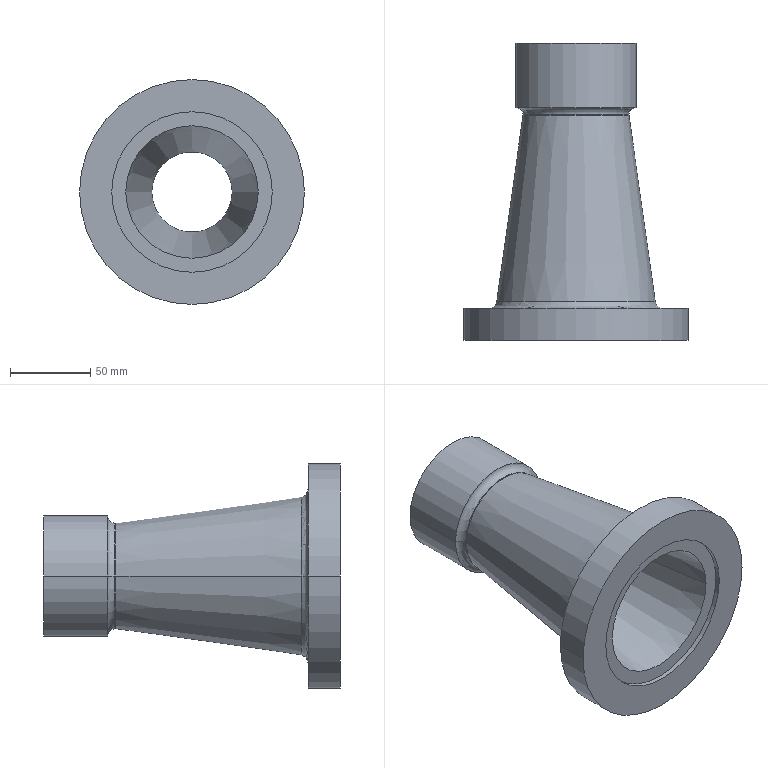Part | SolidWorks | features Revolution 1 | 1 solid | 22 faces | box 140 x 185 x 140 mm | volume 602194 mm3 | cylinder 8 | torus 6 | cone 4 | plane 4 | commonest cylinder face diameters 50 x2 75 x2 100 x2 140 x2
STEP:
#1=CARTESIAN_POINT('',(-37.5,52.5,0.));
#2=VERTEX_POINT('',#1);
#3=CARTESIAN_POINT('',(-33.,48.,0.));
#4=VERTEX_POINT('',#3);
#5=CARTESIAN_POINT('',(-37.5,48.,0.));
#6=DIRECTION('',(0.,0.,-1.));
#7=DIRECTION('',(-1.,0.,0.));
#8=AXIS2_PLACEMENT_3D('',#5,#6,#7);
#9=CIRCLE('',#8,4.5);
#10=EDGE_CURVE('',#2,#4,#9,.T.);
#11=ORIENTED_EDGE('',*,*,#10,.T.);
#12=CARTESIAN_POINT('',(33.,48.,0.));
#13=VERTEX_POINT('',#12);
#14=CARTESIAN_POINT('',(0.,48.,0.));
#15=DIRECTION('',(0.,1.,0.));
#16=DIRECTION('',(-1.,0.,0.));
#17=AXIS2_PLACEMENT_3D('',#14,#15,#16);
#18=CIRCLE('',#17,33.);
#19=EDGE_CURVE('',#4,#13,#18,.T.);
#20=ORIENTED_EDGE('',*,*,#19,.T.);
#21=CARTESIAN_POINT('',(37.5,52.5,0.));
#22=VERTEX_POINT('',#21);
#23=CARTESIAN_POINT('',(37.5,48.,0.));
#24=DIRECTION('',(0.,0.,1.));
#25=DIRECTION('',(1.,0.,0.));
#26=AXIS2_PLACEMENT_3D('',#23,#24,#25);
#27=CIRCLE('',#26,4.5);
#28=EDGE_CURVE('',#22,#13,#27,.T.);
#29=ORIENTED_EDGE('',*,*,#28,.F.);
#30=CARTESIAN_POINT('',(0.,52.5,0.));
#31=DIRECTION('',(0.,1.,0.));
#32=DIRECTION('',(-1.,0.,0.));
#33=AXIS2_PLACEMENT_3D('',#30,#31,#32);
#34=CIRCLE('',#33,37.5);
#35=EDGE_CURVE('',#2,#22,#34,.T.);
#36=ORIENTED_EDGE('',*,*,#35,.F.);
#37=EDGE_LOOP('',(#11,#20,#29,#36));
#38=FACE_OUTER_BOUND('',#37,.T.);
#39=CARTESIAN_POINT('',(0.,48.,0.));
#40=DIRECTION('',(0.,1.,0.));
#41=DIRECTION('',(-1.,0.,0.));
#42=AXIS2_PLACEMENT_3D('',#39,#40,#41);
#43=TOROIDAL_SURFACE('',#42,37.5,4.5);
#44=ADVANCED_FACE('',(#38),#43,.F.);
#45=ORIENTED_EDGE('',*,*,#28,.T.);
#46=CARTESIAN_POINT('',(0.,48.,0.));
#47=DIRECTION('',(0.,1.,0.));
#48=DIRECTION('',(-1.,0.,0.));
#49=AXIS2_PLACEMENT_3D('',#46,#47,#48);
#50=CIRCLE('',#49,33.);
#51=EDGE_CURVE('',#13,#4,#50,.T.);
#52=ORIENTED_EDGE('',*,*,#51,.T.);
#53=ORIENTED_EDGE('',*,*,#10,.F.);
#54=CARTESIAN_POINT('',(0.,52.5,0.));
#55=DIRECTION('',(0.,1.,0.));
#56=DIRECTION('',(-1.,0.,0.));
#57=AXIS2_PLACEMENT_3D('',#54,#55,#56);
#58=CIRCLE('',#57,37.5);
#59=EDGE_CURVE('',#22,#2,#58,.T.);
#60=ORIENTED_EDGE('',*,*,#59,.F.);
#61=EDGE_LOOP('',(#45,#52,#53,#60));
#62=FACE_OUTER_BOUND('',#61,.T.);
#63=CARTESIAN_POINT('',(0.,48.,0.));
#64=DIRECTION('',(0.,1.,0.));
#65=DIRECTION('',(-1.,0.,0.));
#66=AXIS2_PLACEMENT_3D('',#63,#64,#65);
#67=TOROIDAL_SURFACE('',#66,37.5,4.5);
#68=ADVANCED_FACE('',(#62),#67,.F.);
#69=ORIENTED_EDGE('',*,*,#51,.F.);
#70=CARTESIAN_POINT('',(33.044,47.37,0.));
#71=VERTEX_POINT('',#70);
#72=CARTESIAN_POINT('',(37.5,48.,0.));
#73=DIRECTION('',(0.,0.,1.));
#74=DIRECTION('',(1.,0.,0.));
#75=AXIS2_PLACEMENT_3D('',#72,#73,#74);
#76=CIRCLE('',#75,4.5);
#77=EDGE_CURVE('',#13,#71,#76,.T.);
#78=ORIENTED_EDGE('',*,*,#77,.T.);
#79=CARTESIAN_POINT('',(-33.044,47.37,0.));
#80=VERTEX_POINT('',#79);
#81=CARTESIAN_POINT('',(0.,47.37,0.));
#82=DIRECTION('',(0.,1.,0.));
#83=DIRECTION('',(-1.,0.,0.));
#84=AXIS2_PLACEMENT_3D('',#81,#82,#83);
#85=CIRCLE('',#84,33.044);
#86=EDGE_CURVE('',#71,#80,#85,.T.);
#87=ORIENTED_EDGE('',*,*,#86,.T.);
#88=CARTESIAN_POINT('',(-37.5,48.,0.));
#89=DIRECTION('',(0.,0.,-1.));
#90=DIRECTION('',(-1.,0.,0.));
#91=AXIS2_PLACEMENT_3D('',#88,#89,#90);
#92=CIRCLE('',#91,4.5);
#93=EDGE_CURVE('',#4,#80,#92,.T.);
#94=ORIENTED_EDGE('',*,*,#93,.F.);
#95=EDGE_LOOP('',(#69,#78,#87,#94));
#96=FACE_OUTER_BOUND('',#95,.T.);
#97=CARTESIAN_POINT('',(0.,48.,0.));
#98=DIRECTION('',(0.,1.,0.));
#99=DIRECTION('',(-1.,0.,0.));
#100=AXIS2_PLACEMENT_3D('',#97,#98,#99);
#101=TOROIDAL_SURFACE('',#100,37.5,4.5);
#102=ADVANCED_FACE('',(#96),#101,.F.);
#103=CARTESIAN_POINT('',(0.,47.37,0.));
#104=DIRECTION('',(0.,1.,0.));
#105=DIRECTION('',(-1.,0.,0.));
#106=AXIS2_PLACEMENT_3D('',#103,#104,#105);
#107=CIRCLE('',#106,33.044);
#108=EDGE_CURVE('',#80,#71,#107,.T.);
#109=ORIENTED_EDGE('',*,*,#108,.F.);
#110=CARTESIAN_POINT('',(-49.392,-68.2,0.));
#111=VERTEX_POINT('',#110);
#112=CARTESIAN_POINT('',(-49.392,-68.2,0.));
#113=DIRECTION('',(-0.1401,-0.9901,0.));
#114=VECTOR('',#113,1000.);
#115=LINE('',#112,#114);
#116=EDGE_CURVE('',#80,#111,#115,.T.);
#117=ORIENTED_EDGE('',*,*,#116,.T.);
#118=CARTESIAN_POINT('',(49.392,-68.2,0.));
#119=VERTEX_POINT('',#118);
#120=CARTESIAN_POINT('',(0.,-68.2,0.));
#121=DIRECTION('',(0.,1.,0.));
#122=DIRECTION('',(-1.,0.,0.));
#123=AXIS2_PLACEMENT_3D('',#120,#121,#122);
#124=CIRCLE('',#123,49.392);
#125=EDGE_CURVE('',#111,#119,#124,.T.);
#126=ORIENTED_EDGE('',*,*,#125,.T.);
#127=CARTESIAN_POINT('',(49.392,-68.2,0.));
#128=DIRECTION('',(0.1401,-0.9901,0.));
#129=VECTOR('',#128,1000.);
#130=LINE('',#127,#129);
#131=EDGE_CURVE('',#71,#119,#130,.T.);
#132=ORIENTED_EDGE('',*,*,#131,.F.);
#133=EDGE_LOOP('',(#109,#117,#126,#132));
#134=FACE_OUTER_BOUND('',#133,.T.);
#135=CARTESIAN_POINT('',(0.,-68.2,0.));
#136=DIRECTION('',(0.,-1.,0.));
#137=DIRECTION('',(1.,0.,0.));
#138=AXIS2_PLACEMENT_3D('',#135,#136,#137);
#139=CONICAL_SURFACE('',#138,49.392,0.1405);
#140=ADVANCED_FACE('',(#134),#139,.T.);
#141=CARTESIAN_POINT('',(0.,-68.2,0.));
#142=DIRECTION('',(0.,1.,0.));
#143=DIRECTION('',(-1.,0.,0.));
#144=AXIS2_PLACEMENT_3D('',#141,#142,#143);
#145=CIRCLE('',#144,49.392);
#146=EDGE_CURVE('',#119,#111,#145,.T.);
#147=ORIENTED_EDGE('',*,*,#146,.F.);
#148=CARTESIAN_POINT('',(54.343,-72.5,0.));
#149=VERTEX_POINT('',#148);
#150=CARTESIAN_POINT('',(54.343,-67.5,0.));
#151=DIRECTION('',(0.,0.,1.));
#152=DIRECTION('',(1.,0.,0.));
#153=AXIS2_PLACEMENT_3D('',#150,#151,#152);
#154=CIRCLE('',#153,5.);
#155=EDGE_CURVE('',#119,#149,#154,.T.);
#156=ORIENTED_EDGE('',*,*,#155,.T.);
#157=CARTESIAN_POINT('',(-54.343,-72.5,0.));
#158=VERTEX_POINT('',#157);
#159=CARTESIAN_POINT('',(0.,-72.5,0.));
#160=DIRECTION('',(0.,1.,0.));
#161=DIRECTION('',(-1.,0.,0.));
#162=AXIS2_PLACEMENT_3D('',#159,#160,#161);
#163=CIRCLE('',#162,54.343);
#164=EDGE_CURVE('',#149,#158,#163,.T.);
#165=ORIENTED_EDGE('',*,*,#164,.T.);
#166=CARTESIAN_POINT('',(-54.343,-67.5,0.));
#167=DIRECTION('',(0.,0.,-1.));
#168=DIRECTION('',(-1.,0.,0.));
#169=AXIS2_PLACEMENT_3D('',#166,#167,#168);
#170=CIRCLE('',#169,5.);
#171=EDGE_CURVE('',#111,#158,#170,.T.);
#172=ORIENTED_EDGE('',*,*,#171,.F.);
#173=EDGE_LOOP('',(#147,#156,#165,#172));
#174=FACE_OUTER_BOUND('',#173,.T.);
#175=CARTESIAN_POINT('',(0.,-67.5,0.));
#176=DIRECTION('',(0.,1.,0.));
#177=DIRECTION('',(-1.,0.,0.));
#178=AXIS2_PLACEMENT_3D('',#175,#176,#177);
#179=TOROIDAL_SURFACE('',#178,54.343,5.);
#180=ADVANCED_FACE('',(#174),#179,.F.);
#181=CARTESIAN_POINT('',(-70.,-92.5,0.));
#182=VERTEX_POINT('',#181);
#183=CARTESIAN_POINT('',(70.,-92.5,0.));
#184=VERTEX_POINT('',#183);
#185=CARTESIAN_POINT('',(0.,-92.5,0.));
#186=DIRECTION('',(0.,1.,0.));
#187=DIRECTION('',(-1.,0.,0.));
#188=AXIS2_PLACEMENT_3D('',#185,#186,#187);
#189=CIRCLE('',#188,70.);
#190=EDGE_CURVE('',#182,#184,#189,.T.);
#191=ORIENTED_EDGE('',*,*,#190,.T.);
#192=CARTESIAN_POINT('',(70.,-72.5,0.));
#193=VERTEX_POINT('',#192);
#194=CARTESIAN_POINT('',(70.,92.5,0.));
#195=DIRECTION('',(0.,1.,0.));
#196=VECTOR('',#195,1000.);
#197=LINE('',#194,#196);
#198=EDGE_CURVE('',#184,#193,#197,.T.);
#199=ORIENTED_EDGE('',*,*,#198,.T.);
#200=CARTESIAN_POINT('',(-70.,-72.5,0.));
#201=VERTEX_POINT('',#200);
#202=CARTESIAN_POINT('',(0.,-72.5,0.));
#203=DIRECTION('',(0.,1.,0.));
#204=DIRECTION('',(-1.,0.,0.));
#205=AXIS2_PLACEMENT_3D('',#202,#203,#204);
#206=CIRCLE('',#205,70.);
#207=EDGE_CURVE('',#201,#193,#206,.T.);
#208=ORIENTED_EDGE('',*,*,#207,.F.);
#209=CARTESIAN_POINT('',(-70.,92.5,0.));
#210=DIRECTION('',(0.,1.,0.));
#211=VECTOR('',#210,1000.);
#212=LINE('',#209,#211);
#213=EDGE_CURVE('',#182,#201,#212,.T.);
#214=ORIENTED_EDGE('',*,*,#213,.F.);
#215=EDGE_LOOP('',(#191,#199,#208,#214));
#216=FACE_OUTER_BOUND('',#215,.T.);
#217=CARTESIAN_POINT('',(0.,92.5,0.));
#218=DIRECTION('',(0.,1.,0.));
#219=DIRECTION('',(-1.,0.,0.));
#220=AXIS2_PLACEMENT_3D('',#217,#218,#219);
#221=CYLINDRICAL_SURFACE('',#220,70.);
#222=ADVANCED_FACE('',(#216),#221,.T.);
#223=CARTESIAN_POINT('',(50.,-92.5,0.));
#224=VERTEX_POINT('',#223);
#225=CARTESIAN_POINT('',(-50.,-92.5,0.));
#226=VERTEX_POINT('',#225);
#227=CARTESIAN_POINT('',(0.,-92.5,0.));
#228=DIRECTION('',(0.,1.,0.));
#229=DIRECTION('',(-1.,0.,0.));
#230=AXIS2_PLACEMENT_3D('',#227,#228,#229);
#231=CIRCLE('',#230,50.);
#232=EDGE_CURVE('',#224,#226,#231,.T.);
#233=ORIENTED_EDGE('',*,*,#232,.F.);
#234=CARTESIAN_POINT('',(50.,-89.5,0.));
#235=VERTEX_POINT('',#234);
#236=CARTESIAN_POINT('',(50.,92.5,0.));
#237=DIRECTION('',(0.,1.,0.));
#238=VECTOR('',#237,1000.);
#239=LINE('',#236,#238);
#240=EDGE_CURVE('',#224,#235,#239,.T.);
#241=ORIENTED_EDGE('',*,*,#240,.T.);
#242=CARTESIAN_POINT('',(-50.,-89.5,0.));
#243=VERTEX_POINT('',#242);
#244=CARTESIAN_POINT('',(0.,-89.5,0.));
#245=DIRECTION('',(0.,1.,0.));
#246=DIRECTION('',(-1.,0.,0.));
#247=AXIS2_PLACEMENT_3D('',#244,#245,#246);
#248=CIRCLE('',#247,50.);
#249=EDGE_CURVE('',#235,#243,#248,.T.);
#250=ORIENTED_EDGE('',*,*,#249,.T.);
#251=CARTESIAN_POINT('',(-50.,92.5,0.));
#252=DIRECTION('',(0.,1.,0.));
#253=VECTOR('',#252,1000.);
#254=LINE('',#251,#253);
#255=EDGE_CURVE('',#226,#243,#254,.T.);
#256=ORIENTED_EDGE('',*,*,#255,.F.);
#257=EDGE_LOOP('',(#233,#241,#250,#256));
#258=FACE_OUTER_BOUND('',#257,.T.);
#259=CARTESIAN_POINT('',(0.,92.5,0.));
#260=DIRECTION('',(0.,1.,0.));
#261=DIRECTION('',(-1.,0.,0.));
#262=AXIS2_PLACEMENT_3D('',#259,#260,#261);
#263=CYLINDRICAL_SURFACE('',#262,50.);
#264=ADVANCED_FACE('',(#258),#263,.F.);
#265=CARTESIAN_POINT('',(25.,25.7,0.));
#266=VERTEX_POINT('',#265);
#267=CARTESIAN_POINT('',(-25.,25.7,0.));
#268=VERTEX_POINT('',#267);
#269=CARTESIAN_POINT('',(0.,25.7,0.));
#270=DIRECTION('',(0.,1.,0.));
#271=DIRECTION('',(-1.,0.,0.));
#272=AXIS2_PLACEMENT_3D('',#269,#270,#271);
#273=CIRCLE('',#272,25.);
#274=EDGE_CURVE('',#266,#268,#273,.T.);
#275=ORIENTED_EDGE('',*,*,#274,.T.);
#276=CARTESIAN_POINT('',(-41.295,-89.5,0.));
#277=VERTEX_POINT('',#276);
#278=CARTESIAN_POINT('',(-25.,25.7,0.));
#279=DIRECTION('',(-0.1401,-0.9901,0.));
#280=VECTOR('',#279,1000.);
#281=LINE('',#278,#280);
#282=EDGE_CURVE('',#268,#277,#281,.T.);
#283=ORIENTED_EDGE('',*,*,#282,.T.);
#284=CARTESIAN_POINT('',(41.295,-89.5,0.));
#285=VERTEX_POINT('',#284);
#286=CARTESIAN_POINT('',(0.,-89.5,0.));
#287=DIRECTION('',(0.,1.,0.));
#288=DIRECTION('',(-1.,0.,0.));
#289=AXIS2_PLACEMENT_3D('',#286,#287,#288);
#290=CIRCLE('',#289,41.295);
#291=EDGE_CURVE('',#285,#277,#290,.T.);
#292=ORIENTED_EDGE('',*,*,#291,.F.);
#293=CARTESIAN_POINT('',(25.,25.7,0.));
#294=DIRECTION('',(0.1401,-0.9901,0.));
#295=VECTOR('',#294,1000.);
#296=LINE('',#293,#295);
#297=EDGE_CURVE('',#266,#285,#296,.T.);
#298=ORIENTED_EDGE('',*,*,#297,.F.);
#299=EDGE_LOOP('',(#275,#283,#292,#298));
#300=FACE_OUTER_BOUND('',#299,.T.);
#301=CARTESIAN_POINT('',(0.,25.7,0.));
#302=DIRECTION('',(0.,-1.,0.));
#303=DIRECTION('',(1.,0.,0.));
#304=AXIS2_PLACEMENT_3D('',#301,#302,#303);
#305=CONICAL_SURFACE('',#304,25.,0.1405);
#306=ADVANCED_FACE('',(#300),#305,.F.);
#307=ORIENTED_EDGE('',*,*,#274,.F.);
#308=CARTESIAN_POINT('',(25.,92.5,0.));
#309=VERTEX_POINT('',#308);
#310=CARTESIAN_POINT('',(25.,92.5,0.));
#311=DIRECTION('',(0.,1.,0.));
#312=VECTOR('',#311,1000.);
#313=LINE('',#310,#312);
#314=EDGE_CURVE('',#266,#309,#313,.T.);
#315=ORIENTED_EDGE('',*,*,#314,.T.);
#316=CARTESIAN_POINT('',(-25.,92.5,0.));
#317=VERTEX_POINT('',#316);
#318=CARTESIAN_POINT('',(0.,92.5,0.));
#319=DIRECTION('',(0.,1.,0.));
#320=DIRECTION('',(-1.,0.,0.));
#321=AXIS2_PLACEMENT_3D('',#318,#319,#320);
#322=CIRCLE('',#321,25.);
#323=EDGE_CURVE('',#309,#317,#322,.T.);
#324=ORIENTED_EDGE('',*,*,#323,.T.);
#325=CARTESIAN_POINT('',(-25.,92.5,0.));
#326=DIRECTION('',(0.,1.,0.));
#327=VECTOR('',#326,1000.);
#328=LINE('',#325,#327);
#329=EDGE_CURVE('',#268,#317,#328,.T.);
#330=ORIENTED_EDGE('',*,*,#329,.F.);
#331=EDGE_LOOP('',(#307,#315,#324,#330));
#332=FACE_OUTER_BOUND('',#331,.T.);
#333=CARTESIAN_POINT('',(0.,92.5,0.));
#334=DIRECTION('',(0.,1.,0.));
#335=DIRECTION('',(-1.,0.,0.));
#336=AXIS2_PLACEMENT_3D('',#333,#334,#335);
#337=CYLINDRICAL_SURFACE('',#336,25.);
#338=ADVANCED_FACE('',(#332),#337,.F.);
#339=ORIENTED_EDGE('',*,*,#35,.T.);
#340=CARTESIAN_POINT('',(37.5,92.5,0.));
#341=VERTEX_POINT('',#340);
#342=CARTESIAN_POINT('',(37.5,92.5,0.));
#343=DIRECTION('',(0.,1.,0.));
#344=VECTOR('',#343,1000.);
#345=LINE('',#342,#344);
#346=EDGE_CURVE('',#22,#341,#345,.T.);
#347=ORIENTED_EDGE('',*,*,#346,.T.);
#348=CARTESIAN_POINT('',(-37.5,92.5,0.));
#349=VERTEX_POINT('',#348);
#350=CARTESIAN_POINT('',(0.,92.5,0.));
#351=DIRECTION('',(0.,1.,0.));
#352=DIRECTION('',(-1.,0.,0.));
#353=AXIS2_PLACEMENT_3D('',#350,#351,#352);
#354=CIRCLE('',#353,37.5);
#355=EDGE_CURVE('',#349,#341,#354,.T.);
#356=ORIENTED_EDGE('',*,*,#355,.F.);
#357=CARTESIAN_POINT('',(-37.5,92.5,0.));
#358=DIRECTION('',(0.,1.,0.));
#359=VECTOR('',#358,1000.);
#360=LINE('',#357,#359);
#361=EDGE_CURVE('',#2,#349,#360,.T.);
#362=ORIENTED_EDGE('',*,*,#361,.F.);
#363=EDGE_LOOP('',(#339,#347,#356,#362));
#364=FACE_OUTER_BOUND('',#363,.T.);
#365=CARTESIAN_POINT('',(0.,92.5,0.));
#366=DIRECTION('',(0.,1.,0.));
#367=DIRECTION('',(-1.,0.,0.));
#368=AXIS2_PLACEMENT_3D('',#365,#366,#367);
#369=CYLINDRICAL_SURFACE('',#368,37.5);
#370=ADVANCED_FACE('',(#364),#369,.T.);
#371=ORIENTED_EDGE('',*,*,#346,.F.);
#372=ORIENTED_EDGE('',*,*,#59,.T.);
#373=ORIENTED_EDGE('',*,*,#361,.T.);
#374=CARTESIAN_POINT('',(0.,92.5,0.));
#375=DIRECTION('',(0.,1.,0.));
#376=DIRECTION('',(-1.,0.,0.));
#377=AXIS2_PLACEMENT_3D('',#374,#375,#376);
#378=CIRCLE('',#377,37.5);
#379=EDGE_CURVE('',#341,#349,#378,.T.);
#380=ORIENTED_EDGE('',*,*,#379,.F.);
#381=EDGE_LOOP('',(#371,#372,#373,#380));
#382=FACE_OUTER_BOUND('',#381,.T.);
#383=CARTESIAN_POINT('',(0.,92.5,0.));
#384=DIRECTION('',(0.,1.,0.));
#385=DIRECTION('',(-1.,0.,0.));
#386=AXIS2_PLACEMENT_3D('',#383,#384,#385);
#387=CYLINDRICAL_SURFACE('',#386,37.5);
#388=ADVANCED_FACE('',(#382),#387,.T.);
#389=CARTESIAN_POINT('',(0.,92.5,0.));
#390=DIRECTION('',(0.,1.,0.));
#391=DIRECTION('',(-1.,0.,0.));
#392=AXIS2_PLACEMENT_3D('',#389,#390,#391);
#393=CIRCLE('',#392,25.);
#394=EDGE_CURVE('',#317,#309,#393,.T.);
#395=ORIENTED_EDGE('',*,*,#394,.F.);
#396=ORIENTED_EDGE('',*,*,#323,.F.);
#397=EDGE_LOOP('',(#395,#396));
#398=FACE_BOUND('',#397,.T.);
#399=ORIENTED_EDGE('',*,*,#355,.T.);
#400=ORIENTED_EDGE('',*,*,#379,.T.);
#401=EDGE_LOOP('',(#399,#400));
#402=FACE_OUTER_BOUND('',#401,.T.);
#403=CARTESIAN_POINT('',(37.5,92.5,0.));
#404=DIRECTION('',(0.,-1.,0.));
#405=DIRECTION('',(1.,0.,0.));
#406=AXIS2_PLACEMENT_3D('',#403,#404,#405);
#407=PLANE('',#406);
#408=ADVANCED_FACE('',(#398,#402),#407,.F.);
#409=ORIENTED_EDGE('',*,*,#314,.F.);
#410=CARTESIAN_POINT('',(0.,25.7,0.));
#411=DIRECTION('',(0.,1.,0.));
#412=DIRECTION('',(-1.,0.,0.));
#413=AXIS2_PLACEMENT_3D('',#410,#411,#412);
#414=CIRCLE('',#413,25.);
#415=EDGE_CURVE('',#268,#266,#414,.T.);
#416=ORIENTED_EDGE('',*,*,#415,.F.);
#417=ORIENTED_EDGE('',*,*,#329,.T.);
#418=ORIENTED_EDGE('',*,*,#394,.T.);
#419=EDGE_LOOP('',(#409,#416,#417,#418));
#420=FACE_OUTER_BOUND('',#419,.T.);
#421=CARTESIAN_POINT('',(0.,92.5,0.));
#422=DIRECTION('',(0.,1.,0.));
#423=DIRECTION('',(-1.,0.,0.));
#424=AXIS2_PLACEMENT_3D('',#421,#422,#423);
#425=CYLINDRICAL_SURFACE('',#424,25.);
#426=ADVANCED_FACE('',(#420),#425,.F.);
#427=ORIENTED_EDGE('',*,*,#282,.F.);
#428=ORIENTED_EDGE('',*,*,#415,.T.);
#429=ORIENTED_EDGE('',*,*,#297,.T.);
#430=CARTESIAN_POINT('',(0.,-89.5,0.));
#431=DIRECTION('',(0.,1.,0.));
#432=DIRECTION('',(-1.,0.,0.));
#433=AXIS2_PLACEMENT_3D('',#430,#431,#432);
#434=CIRCLE('',#433,41.295);
#435=EDGE_CURVE('',#277,#285,#434,.T.);
#436=ORIENTED_EDGE('',*,*,#435,.F.);
#437=EDGE_LOOP('',(#427,#428,#429,#436));
#438=FACE_OUTER_BOUND('',#437,.T.);
#439=CARTESIAN_POINT('',(0.,25.7,0.));
#440=DIRECTION('',(0.,-1.,0.));
#441=DIRECTION('',(1.,0.,0.));
#442=AXIS2_PLACEMENT_3D('',#439,#440,#441);
#443=CONICAL_SURFACE('',#442,25.,0.1405);
#444=ADVANCED_FACE('',(#438),#443,.F.);
#445=CARTESIAN_POINT('',(0.,-89.5,0.));
#446=DIRECTION('',(0.,1.,0.));
#447=DIRECTION('',(-1.,0.,0.));
#448=AXIS2_PLACEMENT_3D('',#445,#446,#447);
#449=CIRCLE('',#448,50.);
#450=EDGE_CURVE('',#243,#235,#449,.T.);
#451=ORIENTED_EDGE('',*,*,#450,.F.);
#452=ORIENTED_EDGE('',*,*,#249,.F.);
#453=EDGE_LOOP('',(#451,#452));
#454=FACE_OUTER_BOUND('',#453,.T.);
#455=ORIENTED_EDGE('',*,*,#291,.T.);
#456=ORIENTED_EDGE('',*,*,#435,.T.);
#457=EDGE_LOOP('',(#455,#456));
#458=FACE_BOUND('',#457,.T.);
#459=CARTESIAN_POINT('',(50.,-89.5,0.));
#460=DIRECTION('',(0.,1.,0.));
#461=DIRECTION('',(-1.,0.,0.));
#462=AXIS2_PLACEMENT_3D('',#459,#460,#461);
#463=PLANE('',#462);
#464=ADVANCED_FACE('',(#454,#458),#463,.F.);
#465=ORIENTED_EDGE('',*,*,#240,.F.);
#466=CARTESIAN_POINT('',(0.,-92.5,0.));
#467=DIRECTION('',(0.,1.,0.));
#468=DIRECTION('',(-1.,0.,0.));
#469=AXIS2_PLACEMENT_3D('',#466,#467,#468);
#470=CIRCLE('',#469,50.);
#471=EDGE_CURVE('',#226,#224,#470,.T.);
#472=ORIENTED_EDGE('',*,*,#471,.F.);
#473=ORIENTED_EDGE('',*,*,#255,.T.);
#474=ORIENTED_EDGE('',*,*,#450,.T.);
#475=EDGE_LOOP('',(#465,#472,#473,#474));
#476=FACE_OUTER_BOUND('',#475,.T.);
#477=CARTESIAN_POINT('',(0.,92.5,0.));
#478=DIRECTION('',(0.,1.,0.));
#479=DIRECTION('',(-1.,0.,0.));
#480=AXIS2_PLACEMENT_3D('',#477,#478,#479);
#481=CYLINDRICAL_SURFACE('',#480,50.);
#482=ADVANCED_FACE('',(#476),#481,.F.);
#483=ORIENTED_EDGE('',*,*,#190,.F.);
#484=CARTESIAN_POINT('',(0.,-92.5,0.));
#485=DIRECTION('',(0.,1.,0.));
#486=DIRECTION('',(-1.,0.,0.));
#487=AXIS2_PLACEMENT_3D('',#484,#485,#486);
#488=CIRCLE('',#487,70.);
#489=EDGE_CURVE('',#184,#182,#488,.T.);
#490=ORIENTED_EDGE('',*,*,#489,.F.);
#491=EDGE_LOOP('',(#483,#490));
#492=FACE_OUTER_BOUND('',#491,.T.);
#493=ORIENTED_EDGE('',*,*,#471,.T.);
#494=ORIENTED_EDGE('',*,*,#232,.T.);
#495=EDGE_LOOP('',(#493,#494));
#496=FACE_BOUND('',#495,.T.);
#497=CARTESIAN_POINT('',(70.,-92.5,0.));
#498=DIRECTION('',(0.,1.,0.));
#499=DIRECTION('',(-1.,0.,0.));
#500=AXIS2_PLACEMENT_3D('',#497,#498,#499);
#501=PLANE('',#500);
#502=ADVANCED_FACE('',(#492,#496),#501,.F.);
#503=ORIENTED_EDGE('',*,*,#198,.F.);
#504=ORIENTED_EDGE('',*,*,#489,.T.);
#505=ORIENTED_EDGE('',*,*,#213,.T.);
#506=CARTESIAN_POINT('',(0.,-72.5,0.));
#507=DIRECTION('',(0.,1.,0.));
#508=DIRECTION('',(-1.,0.,0.));
#509=AXIS2_PLACEMENT_3D('',#506,#507,#508);
#510=CIRCLE('',#509,70.);
#511=EDGE_CURVE('',#193,#201,#510,.T.);
#512=ORIENTED_EDGE('',*,*,#511,.F.);
#513=EDGE_LOOP('',(#503,#504,#505,#512));
#514=FACE_OUTER_BOUND('',#513,.T.);
#515=CARTESIAN_POINT('',(0.,92.5,0.));
#516=DIRECTION('',(0.,1.,0.));
#517=DIRECTION('',(-1.,0.,0.));
#518=AXIS2_PLACEMENT_3D('',#515,#516,#517);
#519=CYLINDRICAL_SURFACE('',#518,70.);
#520=ADVANCED_FACE('',(#514),#519,.T.);
#521=CARTESIAN_POINT('',(0.,-72.5,0.));
#522=DIRECTION('',(0.,1.,0.));
#523=DIRECTION('',(-1.,0.,0.));
#524=AXIS2_PLACEMENT_3D('',#521,#522,#523);
#525=CIRCLE('',#524,54.343);
#526=EDGE_CURVE('',#158,#149,#525,.T.);
#527=ORIENTED_EDGE('',*,*,#526,.F.);
#528=ORIENTED_EDGE('',*,*,#164,.F.);
#529=EDGE_LOOP('',(#527,#528));
#530=FACE_BOUND('',#529,.T.);
#531=ORIENTED_EDGE('',*,*,#207,.T.);
#532=ORIENTED_EDGE('',*,*,#511,.T.);
#533=EDGE_LOOP('',(#531,#532));
#534=FACE_OUTER_BOUND('',#533,.T.);
#535=CARTESIAN_POINT('',(70.,-72.5,0.));
#536=DIRECTION('',(0.,-1.,0.));
#537=DIRECTION('',(1.,0.,0.));
#538=AXIS2_PLACEMENT_3D('',#535,#536,#537);
#539=PLANE('',#538);
#540=ADVANCED_FACE('',(#530,#534),#539,.F.);
#541=ORIENTED_EDGE('',*,*,#155,.F.);
#542=ORIENTED_EDGE('',*,*,#125,.F.);
#543=ORIENTED_EDGE('',*,*,#171,.T.);
#544=ORIENTED_EDGE('',*,*,#526,.T.);
#545=EDGE_LOOP('',(#541,#542,#543,#544));
#546=FACE_OUTER_BOUND('',#545,.T.);
#547=CARTESIAN_POINT('',(0.,-67.5,0.));
#548=DIRECTION('',(0.,1.,0.));
#549=DIRECTION('',(-1.,0.,0.));
#550=AXIS2_PLACEMENT_3D('',#547,#548,#549);
#551=TOROIDAL_SURFACE('',#550,54.343,5.);
#552=ADVANCED_FACE('',(#546),#551,.F.);
#553=ORIENTED_EDGE('',*,*,#116,.F.);
#554=ORIENTED_EDGE('',*,*,#86,.F.);
#555=ORIENTED_EDGE('',*,*,#131,.T.);
#556=ORIENTED_EDGE('',*,*,#146,.T.);
#557=EDGE_LOOP('',(#553,#554,#555,#556));
#558=FACE_OUTER_BOUND('',#557,.T.);
#559=CARTESIAN_POINT('',(0.,-68.2,0.));
#560=DIRECTION('',(0.,-1.,0.));
#561=DIRECTION('',(1.,0.,0.));
#562=AXIS2_PLACEMENT_3D('',#559,#560,#561);
#563=CONICAL_SURFACE('',#562,49.392,0.1405);
#564=ADVANCED_FACE('',(#558),#563,.T.);
#565=ORIENTED_EDGE('',*,*,#19,.F.);
#566=ORIENTED_EDGE('',*,*,#93,.T.);
#567=ORIENTED_EDGE('',*,*,#108,.T.);
#568=ORIENTED_EDGE('',*,*,#77,.F.);
#569=EDGE_LOOP('',(#565,#566,#567,#568));
#570=FACE_OUTER_BOUND('',#569,.T.);
#571=CARTESIAN_POINT('',(0.,48.,0.));
#572=DIRECTION('',(0.,1.,0.));
#573=DIRECTION('',(-1.,0.,0.));
#574=AXIS2_PLACEMENT_3D('',#571,#572,#573);
#575=TOROIDAL_SURFACE('',#574,37.5,4.5);
#576=ADVANCED_FACE('',(#570),#575,.F.);
#577=CLOSED_SHELL('',(#44,#68,#102,#140,#180,#222,#264,#306,#338,#370,#388,#408,#426,#444,#464,#482,#502,#520,#540,#552,#564,#576));
#578=MANIFOLD_SOLID_BREP('',#577);
#579=CARTESIAN_POINT('',(0.,0.,0.));
#580=DIRECTION('',(0.,0.,1.));
#581=DIRECTION('',(1.,0.,0.));
#582=AXIS2_PLACEMENT_3D('',#579,#580,#581);
#583=(LENGTH_UNIT()NAMED_UNIT(*)SI_UNIT(.MILLI.,.METRE.));
#584=UNCERTAINTY_MEASURE_WITH_UNIT(LENGTH_MEASURE(0.00001),#583,'','');
#585=(NAMED_UNIT(*)PLANE_ANGLE_UNIT()SI_UNIT($,.RADIAN.));
#586=(NAMED_UNIT(*)SI_UNIT($,.STERADIAN.)SOLID_ANGLE_UNIT());
#587=(GEOMETRIC_REPRESENTATION_CONTEXT(3)GLOBAL_UNCERTAINTY_ASSIGNED_CONTEXT((#584))GLOBAL_UNIT_ASSIGNED_CONTEXT((#583,#585,#586))REPRESENTATION_CONTEXT('',''));
#588=ADVANCED_BREP_SHAPE_REPRESENTATION('',(#578,#582),#587);